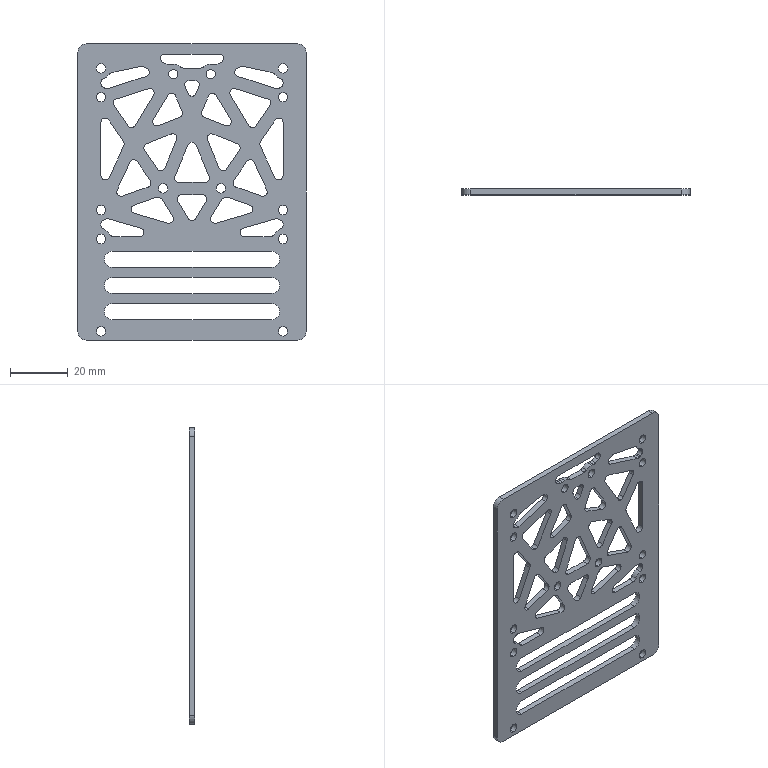Part | SolidWorks | features Fillet 2, Extrusion 1, ICE 1 | 1 solid | 214 faces | box 79 x 2 x 102.5 mm | volume 10788 mm3 | cylinder 139 | plane 75 | commonest cylinder face diameters 3 x87 3.2 x28 7 x14 5.6 x6 6 x4